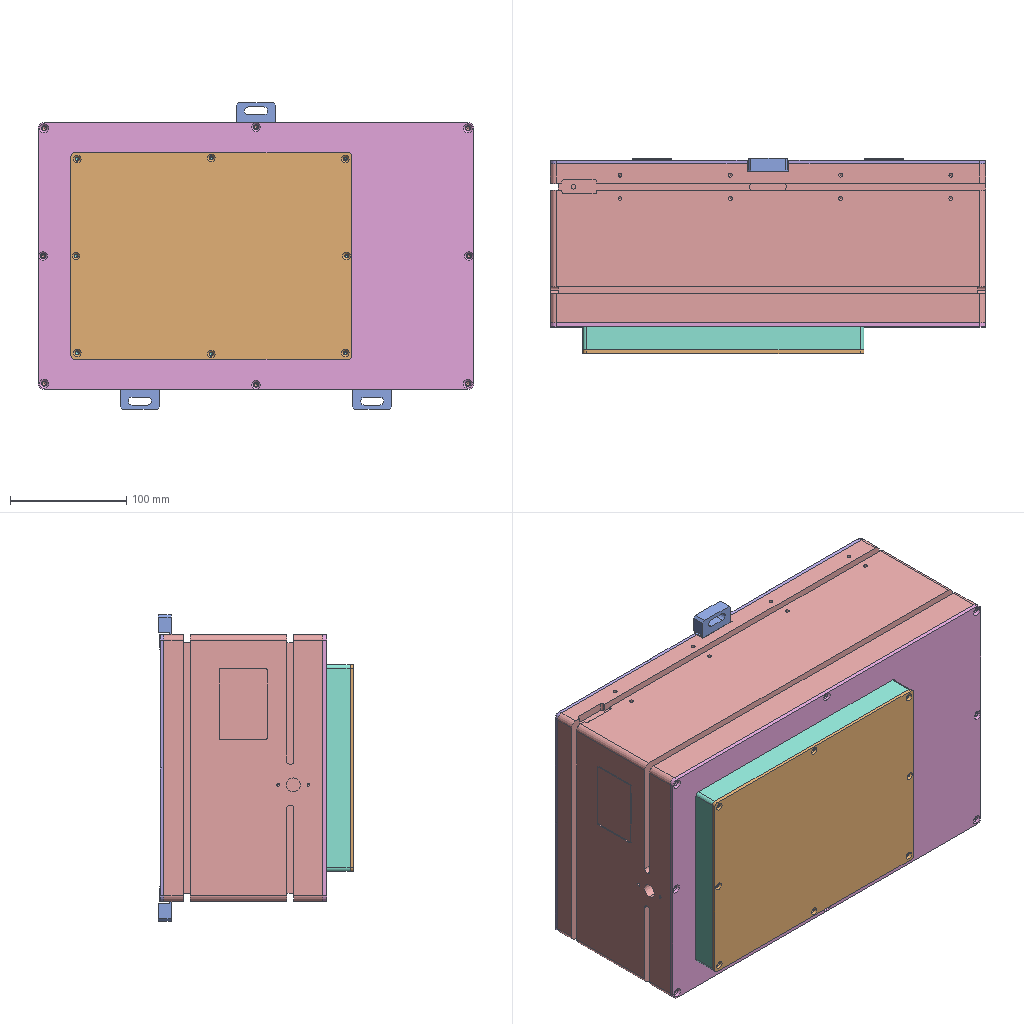Assembly | SolidWorks | 7 different items | 9 placed | box 375 x 168 x 264 mm
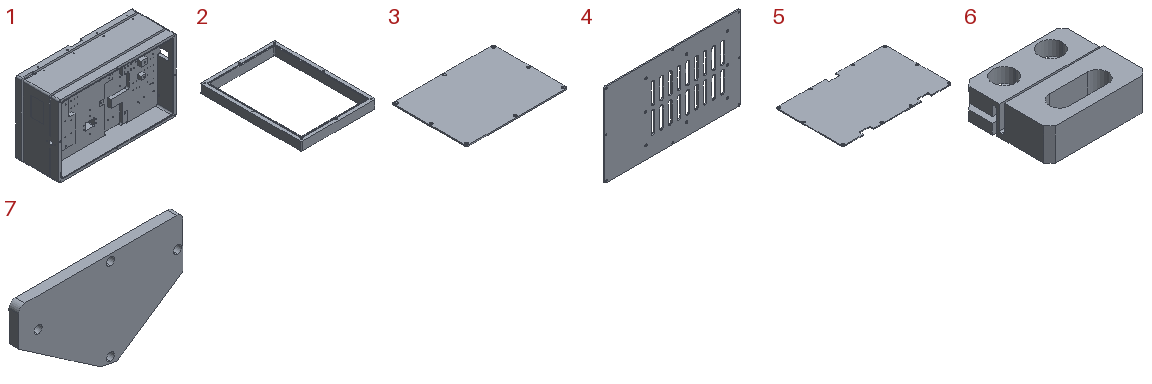Parts list (item | quantity | size | volume | features):
1 | x1 | 375 x 137 x 230 mm | 4002345 mm3 | features ICE 36, HoleWzd 21, Fillet 12, Extrusion 1, SweepCut 1
2 | x1 | 178 x 242 x 20 mm | 172228 mm3 | features MoveFace 4, HoleWzd 2, ICE 2, Extrusion 1, Fillet 1
3 | x1 | 242 x 178 x 3 mm | 128843 mm3 | features Extrusion 1, Fillet 1, HoleWzd 1
4 | x1 | 375 x 3.5 x 230 mm | 264309 mm3 | features HoleWzd 2, MoveFace 2, BaseBody 1, Cut 1
5 | x1 | 375 x 230 x 3 mm | 253484 mm3 | features BaseBody 1, HoleWzd 1, MoveFace 1
6 | x3 | 34 x 29.5 x 11.5 mm | 7154 mm3 | features MoveFace 11, Cut 3, DelFace 2, Fillet 2, BaseBody 1, ICE 1
7 | x1 | 51.5 x 3 x 30.146 mm | 3390 mm3 | features ICE 4, Fillet 2, Cut 1, Extrusion 1, MoveFace 1
Mates (type | each side: item.copy, entity, surface, feature):
Coincident | 1.1 face plane Cut-Extrude1 | 6.1 face plane Input 1
Concentric | 1.1 edge | 6.1 face cylinder Cut-Extrude2
Concentric | 1.1 face cylinder M4 Tapped Hole1 | 6.1 face cylinder Cut-Extrude2
Coincident | 1.1 face plane Cut-Extrude1 | 6.2 face plane Input 1
Concentric | 1.1 edge | 6.2 edge | 2 times
Coincident | 1.1 face plane Cut-Extrude1 | 6.3 face plane Input 1
Concentric | 1.1 face cylinder M4 Tapped Hole1 | 6.3 face cylinder Cut-Extrude1
Concentric | 1.1 edge | 6.3 edge
Coincident | 1.1 face plane Boss-Extrude1 | 4.1 face plane Input 1
Concentric | 1.1 edge | 4.1 edge
Concentric | 1.1 face cylinder M4 Tapped Hole6 | 4.1 edge
Coincident | 2.1 face plane Boss-Extrude1 | 3.1 face plane Boss-Extrude1
Concentric | 2.1 face cone M3 Tapped Hole2 | 3.1 edge | 2 times
Concentric | 4.1 edge | 2.1 face cylinder M3 Tapped Hole1
Concentric | 4.1 edge | 2.1 edge
Coincident | 4.1 face plane Input 1 | 2.1 face plane Boss-Extrude1
Coincident | 1.1 face plane Boss-Extrude1 | 5.1 face plane Input 1
Concentric | 1.1 face cylinder M4 Tapped Hole2 | 5.1 face cone Hole size (% per cross) for half-countersunk slotted wood screw, type 1 | 2 times